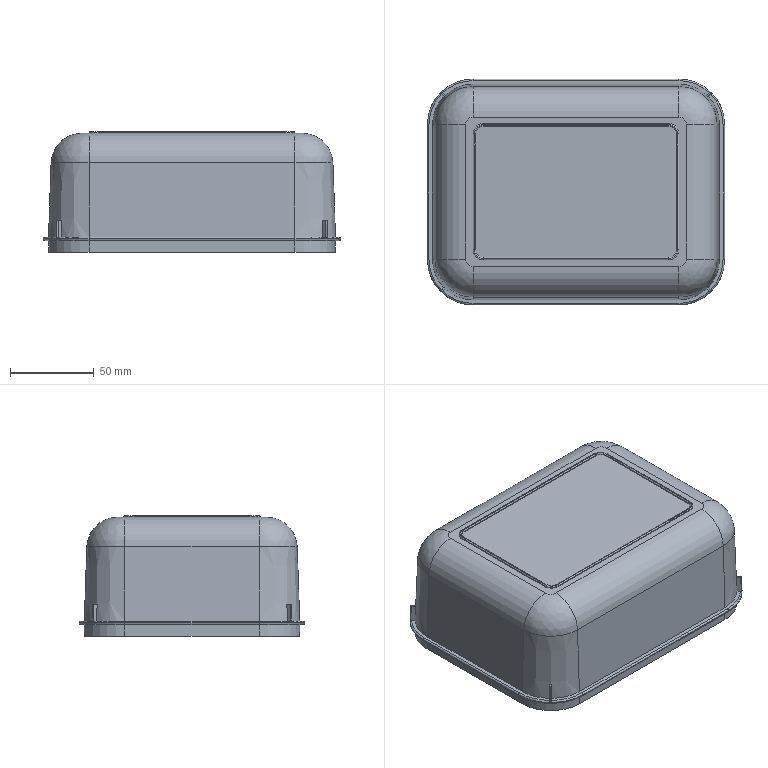Part | STEP file | SL2-MOLD_id710_xmt_txt | 1 solid | 134 faces | box 177.394 x 134.722 x 72.136 mm | volume 76295 mm3 | plane 46 | cylinder 36 | torus 20 | spline 16 | cone 16 | commonest cylinder face diameters 1.219 x8 1.829 x8 9.144 x4 12.192 x4 34.341 x4 36.576 x4